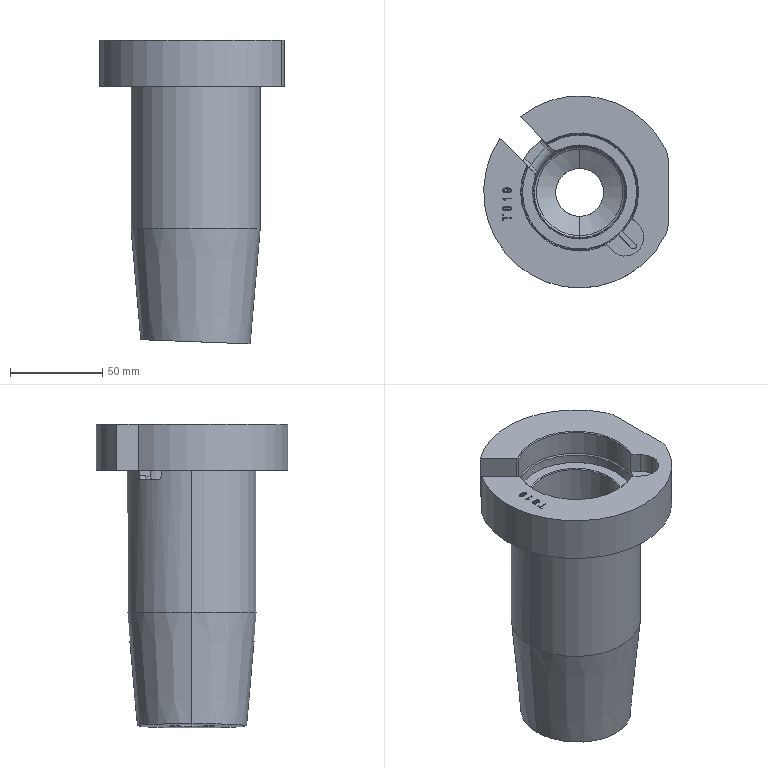Part | Creo | 1 solid | 142 faces | box 100 x 104 x 164.525 mm | volume 382279 mm3 | other 66 | plane 34 | cylinder 22 | cone 9 | spline 6 | torus 5 | commonest cylinder face diameters 4 x6 26 x2 30 x2 50 x2 63 x2 70 x2